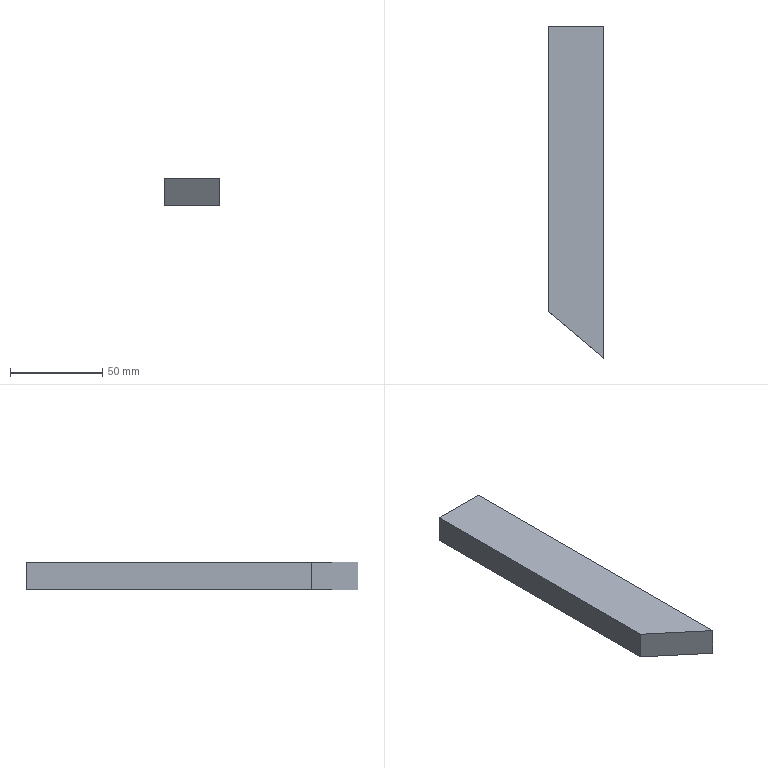Part | NX | features solid 2 | 1 solid | 6 faces | box 30 x 179.583 x 15 mm | volume 75149 mm3 | plane 6
STEP:
#1=CARTESIAN_POINT('',(-103.378,294.27,-15.));
#2=VERTEX_POINT('',#1);
#3=CARTESIAN_POINT('',(-133.378,294.27,-15.));
#4=VERTEX_POINT('',#3);
#5=CARTESIAN_POINT('',(-103.378,294.27,-15.));
#6=DIRECTION('',(1.,0.,0.));
#7=VECTOR('',#6,1000.);
#8=LINE('',#5,#7);
#9=EDGE_CURVE('',#2,#4,#8,.F.);
#10=ORIENTED_EDGE('',*,*,#9,.F.);
#11=CARTESIAN_POINT('',(-103.378,114.687,-15.));
#12=VERTEX_POINT('',#11);
#13=CARTESIAN_POINT('',(-103.378,169.27,-15.));
#14=DIRECTION('',(0.,-1.,0.));
#15=VECTOR('',#14,1000.);
#16=LINE('',#13,#15);
#17=EDGE_CURVE('',#2,#12,#16,.T.);
#18=ORIENTED_EDGE('',*,*,#17,.T.);
#19=CARTESIAN_POINT('',(-133.378,139.86,-15.));
#20=VERTEX_POINT('',#19);
#21=CARTESIAN_POINT('',(-130.255,137.24,-15.));
#22=DIRECTION('',(0.766,-0.6428,0.));
#23=VECTOR('',#22,1000.);
#24=LINE('',#21,#23);
#25=EDGE_CURVE('',#12,#20,#24,.F.);
#26=ORIENTED_EDGE('',*,*,#25,.T.);
#27=CARTESIAN_POINT('',(-133.378,169.27,-15.));
#28=DIRECTION('',(0.,-1.,0.));
#29=VECTOR('',#28,1000.);
#30=LINE('',#27,#29);
#31=EDGE_CURVE('',#4,#20,#30,.T.);
#32=ORIENTED_EDGE('',*,*,#31,.F.);
#33=EDGE_LOOP('',(#10,#18,#26,#32));
#34=FACE_BOUND('',#33,.T.);
#35=CARTESIAN_POINT('',(-103.378,169.27,-15.));
#36=DIRECTION('',(0.,0.,-1.));
#37=DIRECTION('',(0.,-1.,0.));
#38=AXIS2_PLACEMENT_3D('',#35,#36,#37);
#39=PLANE('',#38);
#40=ADVANCED_FACE('',(#34),#39,.T.);
#41=ORIENTED_EDGE('',*,*,#25,.F.);
#42=CARTESIAN_POINT('',(-103.378,114.687,0.));
#43=VERTEX_POINT('',#42);
#44=CARTESIAN_POINT('',(-103.378,114.687,-15.));
#45=DIRECTION('',(0.,0.,-1.));
#46=VECTOR('',#45,1000.);
#47=LINE('',#44,#46);
#48=EDGE_CURVE('',#12,#43,#47,.F.);
#49=ORIENTED_EDGE('',*,*,#48,.T.);
#50=CARTESIAN_POINT('',(-133.378,139.86,0.));
#51=VERTEX_POINT('',#50);
#52=CARTESIAN_POINT('',(-83.587,98.08,0.));
#53=DIRECTION('',(-0.766,0.6428,0.));
#54=VECTOR('',#53,1000.);
#55=LINE('',#52,#54);
#56=EDGE_CURVE('',#43,#51,#55,.T.);
#57=ORIENTED_EDGE('',*,*,#56,.T.);
#58=CARTESIAN_POINT('',(-133.378,139.86,-15.));
#59=DIRECTION('',(0.,0.,-1.));
#60=VECTOR('',#59,1000.);
#61=LINE('',#58,#60);
#62=EDGE_CURVE('',#20,#51,#61,.F.);
#63=ORIENTED_EDGE('',*,*,#62,.F.);
#64=EDGE_LOOP('',(#41,#49,#57,#63));
#65=FACE_BOUND('',#64,.T.);
#66=CARTESIAN_POINT('',(-83.587,98.08,-30.));
#67=DIRECTION('',(0.6428,0.766,0.));
#68=DIRECTION('',(-0.766,0.6428,0.));
#69=AXIS2_PLACEMENT_3D('',#66,#67,#68);
#70=PLANE('',#69);
#71=ADVANCED_FACE('',(#65),#70,.F.);
#72=ORIENTED_EDGE('',*,*,#56,.F.);
#73=CARTESIAN_POINT('',(-103.378,294.27,0.));
#74=VERTEX_POINT('',#73);
#75=CARTESIAN_POINT('',(-103.378,169.27,0.));
#76=DIRECTION('',(0.,-1.,0.));
#77=VECTOR('',#76,1000.);
#78=LINE('',#75,#77);
#79=EDGE_CURVE('',#74,#43,#78,.T.);
#80=ORIENTED_EDGE('',*,*,#79,.F.);
#81=CARTESIAN_POINT('',(-133.378,294.27,0.));
#82=VERTEX_POINT('',#81);
#83=CARTESIAN_POINT('',(-103.378,294.27,0.));
#84=DIRECTION('',(-1.,0.,0.));
#85=VECTOR('',#84,1000.);
#86=LINE('',#83,#85);
#87=EDGE_CURVE('',#74,#82,#86,.T.);
#88=ORIENTED_EDGE('',*,*,#87,.T.);
#89=CARTESIAN_POINT('',(-133.378,169.27,0.));
#90=DIRECTION('',(0.,-1.,0.));
#91=VECTOR('',#90,1000.);
#92=LINE('',#89,#91);
#93=EDGE_CURVE('',#82,#51,#92,.T.);
#94=ORIENTED_EDGE('',*,*,#93,.T.);
#95=EDGE_LOOP('',(#72,#80,#88,#94));
#96=FACE_BOUND('',#95,.T.);
#97=CARTESIAN_POINT('',(-103.378,169.27,0.));
#98=DIRECTION('',(0.,0.,-1.));
#99=DIRECTION('',(0.,-1.,0.));
#100=AXIS2_PLACEMENT_3D('',#97,#98,#99);
#101=PLANE('',#100);
#102=ADVANCED_FACE('',(#96),#101,.F.);
#103=ORIENTED_EDGE('',*,*,#93,.F.);
#104=CARTESIAN_POINT('',(-133.378,294.27,-15.));
#105=DIRECTION('',(0.,0.,-1.));
#106=VECTOR('',#105,1000.);
#107=LINE('',#104,#106);
#108=EDGE_CURVE('',#4,#82,#107,.F.);
#109=ORIENTED_EDGE('',*,*,#108,.F.);
#110=ORIENTED_EDGE('',*,*,#31,.T.);
#111=ORIENTED_EDGE('',*,*,#62,.T.);
#112=EDGE_LOOP('',(#103,#109,#110,#111));
#113=FACE_BOUND('',#112,.T.);
#114=CARTESIAN_POINT('',(-133.378,169.27,-15.));
#115=DIRECTION('',(-1.,0.,0.));
#116=DIRECTION('',(0.,-1.,0.));
#117=AXIS2_PLACEMENT_3D('',#114,#115,#116);
#118=PLANE('',#117);
#119=ADVANCED_FACE('',(#113),#118,.T.);
#120=CARTESIAN_POINT('',(-103.378,294.27,-15.));
#121=DIRECTION('',(0.,0.,-1.));
#122=VECTOR('',#121,1000.);
#123=LINE('',#120,#122);
#124=EDGE_CURVE('',#2,#74,#123,.F.);
#125=ORIENTED_EDGE('',*,*,#124,.F.);
#126=ORIENTED_EDGE('',*,*,#9,.T.);
#127=ORIENTED_EDGE('',*,*,#108,.T.);
#128=ORIENTED_EDGE('',*,*,#87,.F.);
#129=EDGE_LOOP('',(#125,#126,#127,#128));
#130=FACE_BOUND('',#129,.T.);
#131=CARTESIAN_POINT('',(-103.378,294.27,-15.));
#132=DIRECTION('',(0.,-1.,0.));
#133=DIRECTION('',(0.,0.,1.));
#134=AXIS2_PLACEMENT_3D('',#131,#132,#133);
#135=PLANE('',#134);
#136=ADVANCED_FACE('',(#130),#135,.F.);
#137=ORIENTED_EDGE('',*,*,#79,.T.);
#138=ORIENTED_EDGE('',*,*,#48,.F.);
#139=ORIENTED_EDGE('',*,*,#17,.F.);
#140=ORIENTED_EDGE('',*,*,#124,.T.);
#141=EDGE_LOOP('',(#137,#138,#139,#140));
#142=FACE_BOUND('',#141,.T.);
#143=CARTESIAN_POINT('',(-103.378,169.27,-15.));
#144=DIRECTION('',(-1.,0.,0.));
#145=DIRECTION('',(0.,-1.,0.));
#146=AXIS2_PLACEMENT_3D('',#143,#144,#145);
#147=PLANE('',#146);
#148=ADVANCED_FACE('',(#142),#147,.F.);
#149=CLOSED_SHELL('',(#40,#71,#102,#119,#136,#148));
#150=MANIFOLD_SOLID_BREP('',#149);
#151=(LENGTH_UNIT()NAMED_UNIT(*)SI_UNIT(.MILLI.,.METRE.));
#152=UNCERTAINTY_MEASURE_WITH_UNIT(LENGTH_MEASURE(0.00001),#151,'','');
#153=(NAMED_UNIT(*)PLANE_ANGLE_UNIT()SI_UNIT($,.RADIAN.));
#154=(NAMED_UNIT(*)SI_UNIT($,.STERADIAN.)SOLID_ANGLE_UNIT());
#155=(GEOMETRIC_REPRESENTATION_CONTEXT(3)GLOBAL_UNCERTAINTY_ASSIGNED_CONTEXT((#152))GLOBAL_UNIT_ASSIGNED_CONTEXT((#151,#153,#154))REPRESENTATION_CONTEXT('',''));
#156=ADVANCED_BREP_SHAPE_REPRESENTATION('',(#150),#155);